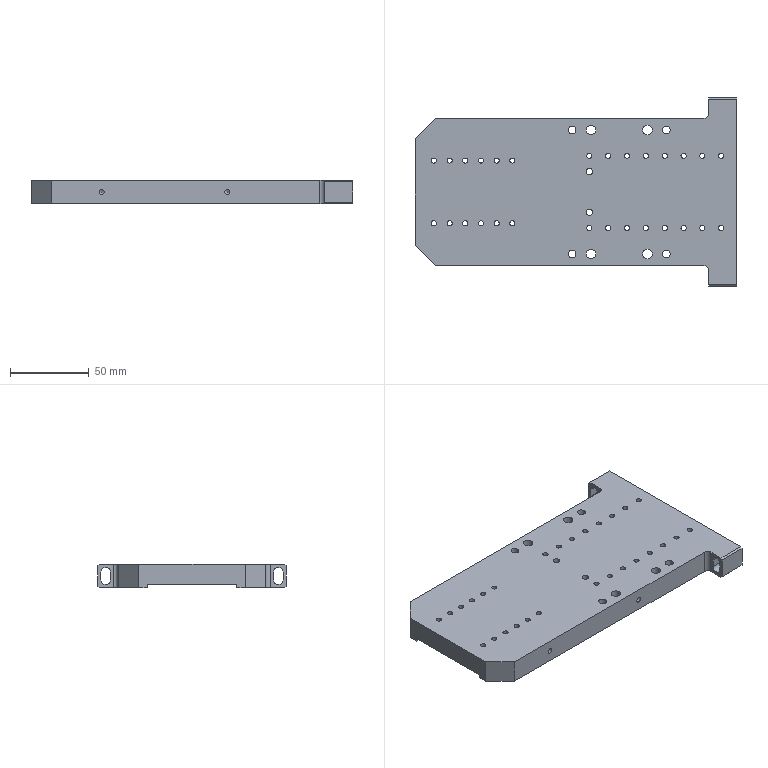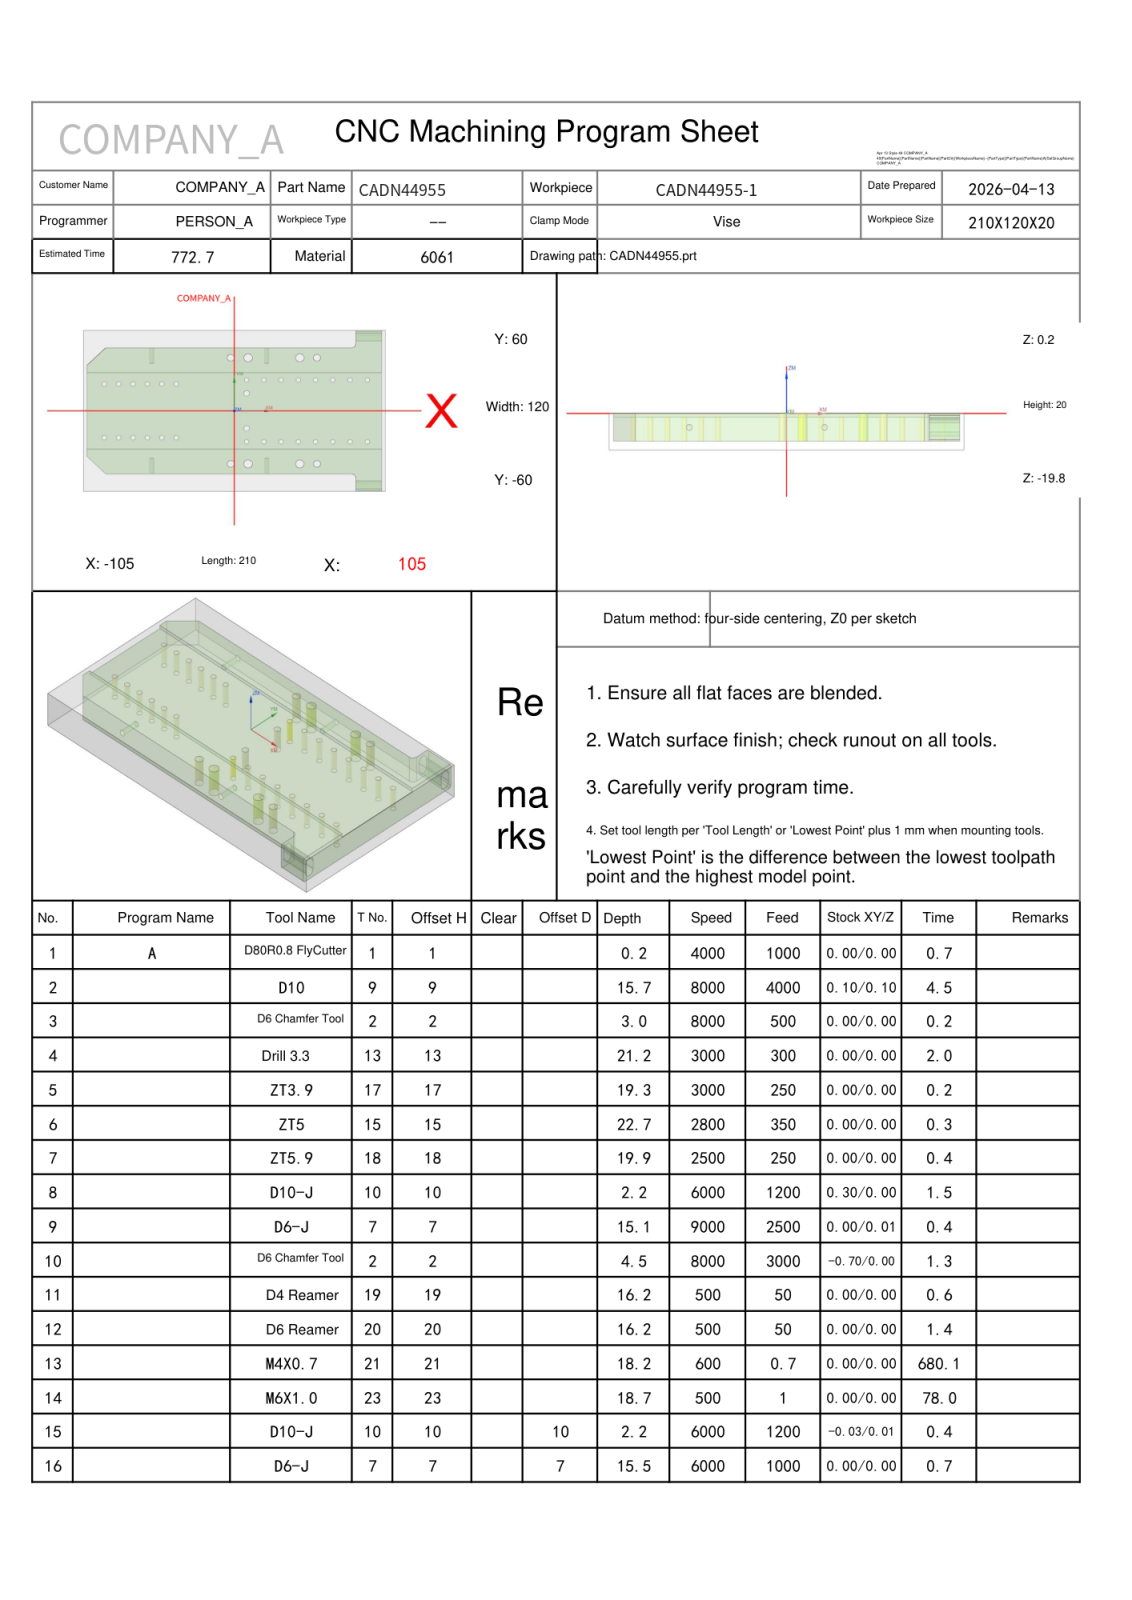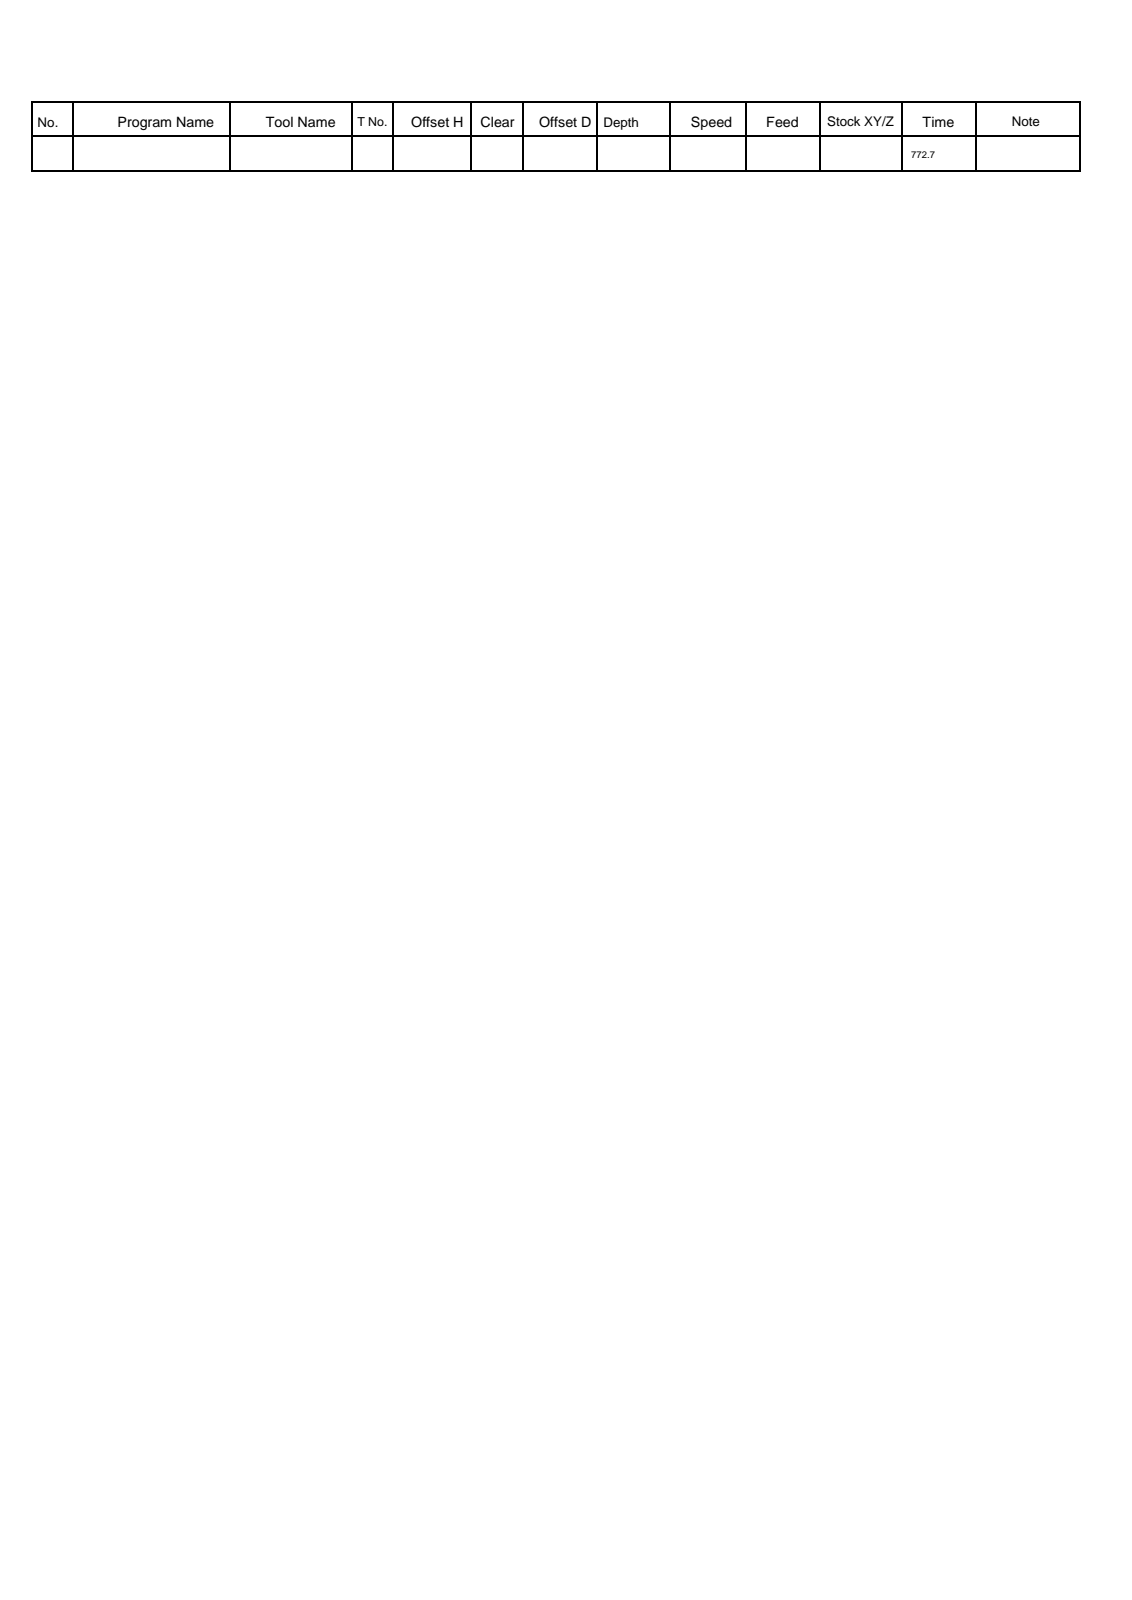NC program | NX | posted by the shop | part box 205 x 120 x 15 mm
Lines 4340 to 4760 of 4760:
N10 T02 M06
(D6 ChamferTool  D=6. R=0. H=02 ce=0.00 di=0.00)
(MAX_Z=20. MIN_Z=-4.3 Time=1.20M)
G00 G90 G54 X83.293 Y-59.461 M03 S8000
G43 H02 Z20.
M08
Z2.935
G01 Z-1.5 F3000.
X83.233 Y-59.289
X83.2 Y-59.
Y-50.
G03 X81.5 Y-48.3 I-1.7 J0.0
G01 X-89.5
X-89.754 Y-48.275
X-89.997 Y-48.201
X-90.222 Y-48.081
X-90.419 Y-47.919
X-103.419 Y-34.919
X-103.581 Y-34.722
X-103.701 Y-34.497
X-103.775 Y-34.254
X-103.8 Y-34.
Y-28.5
G02 X-102.5 Y-27.2 I1.3 J0.0
G01 X0.0
X102.5
G02 X103.8 Y-28.5 I0.0 J-1.3
G01 Y-59.
X103.767 Y-59.289
X103.707 Y-59.461
Z2.935
G00 Z20.
Y59.461
Z2.935
G01 Z-1.5
X103.767 Y59.289
X103.8 Y59.
Y28.5
G02 X102.5 Y27.2 I-1.3 J0.0
G01 X0.0
X-102.5
G02 X-103.8 Y28.5 I0.0 J1.3
G01 Y34.
X-103.775 Y34.254
X-103.701 Y34.497
X-103.581 Y34.722
X-103.419 Y34.919
X-90.419 Y47.919
X-90.222 Y48.081
X-89.997 Y48.201
X-89.754 Y48.275
X-89.5 Y48.3
X81.5
G03 X83.2 Y50. I0.0 J1.7
G01 Y59.
X83.233 Y59.289
X83.293 Y59.461
Z2.935
G00 Z20.
X-104.628 Y-25.465
Z1.755
G01 Z-3.5
G03 X-104.328 Y-25.546 I.3 J.52
X-103.808 Y-25.246 I0.0 J.6
G01 X-103.8 Y-25.216
Y25.216
X-103.808 Y25.246
G03 X-104.328 Y25.546 I-.52 J-.3
X-104.628 Y25.465 I0.0 J-.6
G01 Z1.755
G00 Z20.
X104.628
Z1.755
G01 Z-3.5
G03 X104.328 Y25.546 I-.3 J-.52
X103.808 Y25.246 I0.0 J-.6
G01 X103.8 Y25.216
Y-25.216
X103.808 Y-25.246
G03 X104.328 Y-25.546 I.52 J.3
X104.628 Y-25.465 I0.0 J.6
G01 Z1.755
G00 Z20.
G00 G90 X-40.5 Y20. M03 S8000
Z20.
G98 G81 X-40.5 Y20. Z-4.2 R1. F500.
X-50.5
X-60.5
X-70.5
X-80.5
X-90.5
Y-20.
X-80.5
X-70.5
X-60.5
X-50.5
X-40.5
X8.5 Y-23.
X20.5
X32.5
X44.5
X56.5
X68.5
X80.5
X92.5
Y23.
X80.5
X68.5
X56.5
X44.5
X32.5
X20.5
X8.5
G80
G00 Z20.
G00 G90 X8.5 Y-13. M03 S8000
Z20.
G98 G81 X8.5 Y-13. Z-4.3 R1. F500.
Y13.
G80
G00 Z20.
G00 G90 X57.909 Y-40.521 M03 S8000
Z20.
Z-.6
G01 Z-1.1 F500.
X58.1 Y-41.
G03 X59.6 Y-39.5 I0.0 J1.5
X57.5 Y-37.4 I-2.1 J0.0
X55.4 Y-39.5 I0.0 J-2.1
X57.5 Y-41.6 I2.1 J0.0
X59.6 Y-39.5 I0.0 J2.1
X58.1 Y-38. I-1.5 J0.0
G01 X57.909 Y-38.479
Z-.6
G00 Z20.
X-2.091 Y-40.521
Z-.6
G01 Z-1.1
X-1.9 Y-41.
G03 X-.4 Y-39.5 I0.0 J1.5
X-2.5 Y-37.4 I-2.1 J0.0
X-4.6 Y-39.5 I0.0 J-2.1
X-2.5 Y-41.6 I2.1 J0.0
X-.4 Y-39.5 I0.0 J2.1
X-1.9 Y-38. I-1.5 J0.0
G01 X-2.091 Y-38.479
Z-.6
G00 Z20.
Y38.479
Z-.6
G01 Z-1.1
X-1.9 Y38.
G03 X-.4 Y39.5 I0.0 J1.5
X-2.5 Y41.6 I-2.1 J0.0
X-4.6 Y39.5 I0.0 J-2.1
X-2.5 Y37.4 I2.1 J0.0
X-.4 Y39.5 I0.0 J2.1
X-1.9 Y41. I-1.5 J0.0
G01 X-2.091 Y40.521
Z-.6
G00 Z20.
X57.909 Y38.479
Z-.6
G01 Z-1.1
X58.1 Y38.
G03 X59.6 Y39.5 I0.0 J1.5
X57.5 Y41.6 I-2.1 J0.0
X55.4 Y39.5 I0.0 J-2.1
X57.5 Y37.4 I2.1 J0.0
X59.6 Y39.5 I0.0 J2.1
X58.1 Y41. I-1.5 J0.0
G01 X57.909 Y40.521
Z-.6
G00 Z20.
G00 G90 X46.112 Y-40.647 M03 S8000
Z20.
Z-.5
G01 Z-1. F500.
X46.3 Y-41.
G03 X47.8 Y-39.5 I0.0 J1.5
X45.5 Y-37.2 I-2.3 J0.0
X43.2 Y-39.5 I0.0 J-2.3
X45.5 Y-41.8 I2.3 J0.0
X47.8 Y-39.5 I0.0 J2.3
X46.3 Y-38. I-1.5 J0.0
G01 X46.112 Y-38.353
Z-.5
G00 Z20.
X10.112 Y-40.647
Z-.5
G01 Z-1.
X10.3 Y-41.
G03 X11.8 Y-39.5 I0.0 J1.5
X9.5 Y-37.2 I-2.3 J0.0
X7.2 Y-39.5 I0.0 J-2.3
X9.5 Y-41.8 I2.3 J0.0
X11.8 Y-39.5 I0.0 J2.3
X10.3 Y-38. I-1.5 J0.0
G01 X10.112 Y-38.353
Z-.5
G00 Z20.
Y38.353
Z-.5
G01 Z-1.
X10.3 Y38.
G03 X11.8 Y39.5 I0.0 J1.5
X9.5 Y41.8 I-2.3 J0.0
X7.2 Y39.5 I0.0 J-2.3
X9.5 Y37.2 I2.3 J0.0
X11.8 Y39.5 I0.0 J2.3
X10.3 Y41. I-1.5 J0.0
G01 X10.112 Y40.647
Z-.5
G00 Z20.
X46.112 Y38.353
Z-.5
G01 Z-1.
X46.3 Y38.
G03 X47.8 Y39.5 I0.0 J1.5
X45.5 Y41.8 I-2.3 J0.0
X43.2 Y39.5 I0.0 J-2.3
X45.5 Y37.2 I2.3 J0.0
X47.8 Y39.5 I0.0 J2.3
X46.3 Y41. I-1.5 J0.0
G01 X46.112 Y40.647
Z-.5
G00 Z20.
G00 G90 X105.4 Y-60.708 M03 S6500
Z20.
Z-.2
G01 Z-1.7 F1500.
X105.332 Y-60.699
X105.263 Y-60.7
X81.737
X81.668 Y-60.699
X81.6 Y-60.708
Z-.2
G00 Z20.
Y60.708
Z-.2
G01 Z-1.7
X81.668 Y60.699
X81.737 Y60.7
X105.263
X105.332 Y60.699
X105.4 Y60.708
Z-.2
G00 Z20.
G91 G28 Z0.0
M05
M09
G91 G28 Z0.0
M01
N11 T19 M06
(D4 Reamer D=4. DR_a=180 H=19)
(MAX_Z=20. MIN_Z=-16. Time=0.61M)
G00 G90 G54 X8.5 Y-13. M03 S500
G43 H19 Z20.
M08
G98 G81 X8.5 Y-13. Z-16. R-1. F50.
Y13.
G80
G00 Z20.
G91 G28 Z0.0
M05
M09
G91 G28 Z0.0
M01
N12 T20 M06
(D6 Reamer D=6. DR_a=180 H=20)
(MAX_Z=20. MIN_Z=-16. Time=1.38M)
G00 G90 G54 X45.5 Y-39.5 M03 S500
G43 H20 Z20.
M08
G98 G81 X45.5 Y-39.5 Z-16. R1. F50.
X9.5
Y39.5
X45.5
G80
G00 Z20.
G91 G28 Z0.0
M05
M09
G91 G28 Z0.0
M01
N13 T21 M06
(M4X0.7 D=3.3 DR_a=180 H=21)
(MAX_Z=20. MIN_Z=-18. Time=1320.04M)
G00 G90 G54 X-40.5 Y20. M03 S600
G43 H21 Z20.
M08
G95
/M29
G98 G84 X-40.5 Y20. Z-18. R-1. F.7 Q4.
X-50.5
X-60.5
X-70.5
X-80.5
X-90.5
Y-20.
X-80.5
X-70.5
X-60.5
X-50.5
X-40.5
X8.5 Y-23.
X20.5
X32.5
X44.5
X56.5
X68.5
X80.5
X92.5
Y23.
X80.5
X68.5
X56.5
X44.5
X32.5
X20.5
X8.5
G80
G94
G00 Z20.
G91 G28 Z0.0
M05
M09
G91 G28 Z0.0
M01
N14 T23 M06
(M6X1.0 D=5. DR_a=180 H=23)
(MAX_Z=20. MIN_Z=-18.5 Time=152.02M)
G00 G90 G54 X57.5 Y-39.5 M03 S500
G43 H23 Z20.
M08
G95
/M29
G98 G84 X57.5 Y-39.5 Z-18.5 R1. F1. Q3.
X-2.5
Y39.5
X57.5
G80
G94
G00 Z20.
G91 G28 Z0.0
M05
M09
G91 G28 Z0.0
M01
N15 T10 M06
(D10-J  D=10. R=0. H=10 ce=-0.03 di=0.01)
(D.N=10 MAX_Z=20. MIN_Z=-2. Time=0.38M)
G00 G90 G54 X-108. Y-22.43 M03 S6000
G43 H10 Z20.
M08
Z-1.495
G01 Z-1.995 F1200.
G41 D10
Y-22.53
G03 X-107. Y-23.53 I1. J0.0
G01 X107.
G03 X108. Y-22.53 I0.0 J1.
G01 G40 Y-22.43
Z-1.495
G00 Z20.
Y22.43
Z-1.495
G01 Z-1.995
G41 D10
Y22.53
G03 X107. Y23.53 I-1. J0.0
G01 X-107.
G03 X-108. Y22.53 I0.0 J-1.
G01 G40 Y22.43
Z-1.495
G00 Z20.
G91 G28 Z0.0
M05
M09
G91 G28 Z0.0
M01
N16 T07 M06
(D6-J  D=6. R=0. H=07 ce=0.00 di=0.00)
(D.N=07 MAX_Z=20. MIN_Z=-15.3 Time=0.66M)
G00 G90 G54 X-90.517 Y51.073 M03 S6000
G43 H07 Z20.
M08
Z-14.8
G01 Z-15.3 F1000.
G41 D07
X-90.492 Y50.875
G03 X-89.5 Y50. I.992 J.125
G01 X81.5
Y60.
G02 X84.5 Y63. I3. J0.0
G01 X102.5
G02 X105.5 Y60. I0.0 J-3.
G01 Y-60.
G02 X102.5 Y-63. I-3. J0.0
G01 X84.5
G02 X81.5 Y-60. I0.0 J3.
G01 Y-50.
X-89.5
G02 X-91.621 Y-49.121 I0.0 J3.
G01 X-104.621 Y-36.121
G02 X-105.5 Y-34. I2.121 J2.121
G01 Y34.
G02 X-104.621 Y36.121 I3. J0.0
G01 X-91.621 Y49.121
G02 X-89.5 Y50. I2.121 J-2.121
G01 X-89.
G03 X-88. Y51. I0.0 J1.
G01 G40 Y51.2
Z-14.8
G00 Z20.
M05
M09
G91 G28 Z0.0
G91 G28 Y0.0
M30
%